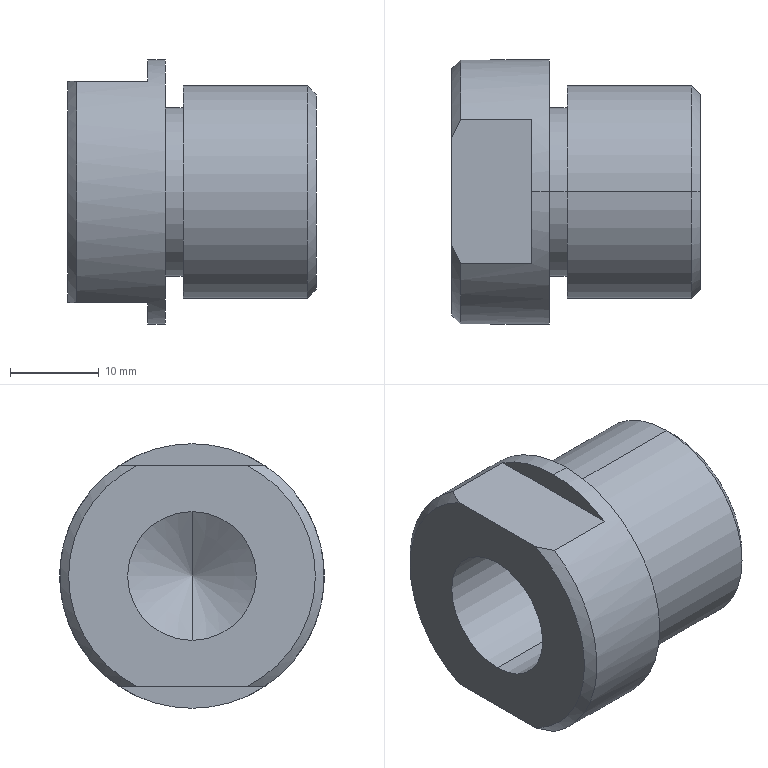Part | SolidWorks | features BaseBody 1 | 1 solid | 22 faces | box 28 x 29.8 x 29.8 mm | volume 11601 mm3 | cylinder 8 | plane 8 | cone 6 | commonest cylinder face diameters 14.5 x2 19 x2 24 x2 29.8 x2
STEP:
#1=CARTESIAN_POINT('',(27.,0.,12.));
#2=VERTEX_POINT('',#1);
#3=CARTESIAN_POINT('',(27.,0.,-12.));
#4=VERTEX_POINT('',#3);
#5=CARTESIAN_POINT('',(27.,0.,0.));
#6=DIRECTION('',(-1.,0.,0.));
#7=DIRECTION('',(0.,0.,1.));
#8=AXIS2_PLACEMENT_3D('',#5,#6,#7);
#9=CIRCLE('',#8,12.);
#10=EDGE_CURVE('',#2,#4,#9,.T.);
#11=ORIENTED_EDGE('',*,*,#10,.T.);
#12=CARTESIAN_POINT('',(13.,0.,-12.));
#13=VERTEX_POINT('',#12);
#14=CARTESIAN_POINT('',(0.,0.,-12.));
#15=DIRECTION('',(-1.,0.,0.));
#16=VECTOR('',#15,1000.);
#17=LINE('',#14,#16);
#18=EDGE_CURVE('',#4,#13,#17,.T.);
#19=ORIENTED_EDGE('',*,*,#18,.T.);
#20=CARTESIAN_POINT('',(13.,0.,12.));
#21=VERTEX_POINT('',#20);
#22=CARTESIAN_POINT('',(13.,0.,0.));
#23=DIRECTION('',(1.,0.,0.));
#24=DIRECTION('',(0.,0.,1.));
#25=AXIS2_PLACEMENT_3D('',#22,#23,#24);
#26=CIRCLE('',#25,12.);
#27=EDGE_CURVE('',#13,#21,#26,.T.);
#28=ORIENTED_EDGE('',*,*,#27,.T.);
#29=CARTESIAN_POINT('',(0.,0.,12.));
#30=DIRECTION('',(-1.,0.,0.));
#31=VECTOR('',#30,1000.);
#32=LINE('',#29,#31);
#33=EDGE_CURVE('',#2,#21,#32,.T.);
#34=ORIENTED_EDGE('',*,*,#33,.F.);
#35=EDGE_LOOP('',(#11,#19,#28,#34));
#36=FACE_OUTER_BOUND('',#35,.T.);
#37=CARTESIAN_POINT('',(0.,0.,0.));
#38=DIRECTION('',(-1.,0.,0.));
#39=DIRECTION('',(0.,0.,1.));
#40=AXIS2_PLACEMENT_3D('',#37,#38,#39);
#41=CYLINDRICAL_SURFACE('',#40,12.);
#42=ADVANCED_FACE('',(#36),#41,.T.);
#43=CARTESIAN_POINT('',(28.,0.,11.));
#44=VERTEX_POINT('',#43);
#45=CARTESIAN_POINT('',(28.,0.,-11.));
#46=VERTEX_POINT('',#45);
#47=CARTESIAN_POINT('',(28.,0.,0.));
#48=DIRECTION('',(-1.,0.,0.));
#49=DIRECTION('',(0.,0.,1.));
#50=AXIS2_PLACEMENT_3D('',#47,#48,#49);
#51=CIRCLE('',#50,11.);
#52=EDGE_CURVE('',#44,#46,#51,.T.);
#53=ORIENTED_EDGE('',*,*,#52,.T.);
#54=CARTESIAN_POINT('',(27.,0.,-12.));
#55=DIRECTION('',(-0.7071,0.,-0.7071));
#56=VECTOR('',#55,1000.);
#57=LINE('',#54,#56);
#58=EDGE_CURVE('',#46,#4,#57,.T.);
#59=ORIENTED_EDGE('',*,*,#58,.T.);
#60=ORIENTED_EDGE('',*,*,#10,.F.);
#61=CARTESIAN_POINT('',(27.,0.,12.));
#62=DIRECTION('',(-0.7071,0.,0.7071));
#63=VECTOR('',#62,1000.);
#64=LINE('',#61,#63);
#65=EDGE_CURVE('',#44,#2,#64,.T.);
#66=ORIENTED_EDGE('',*,*,#65,.F.);
#67=EDGE_LOOP('',(#53,#59,#60,#66));
#68=FACE_OUTER_BOUND('',#67,.T.);
#69=CARTESIAN_POINT('',(27.,0.,0.));
#70=DIRECTION('',(-1.,0.,0.));
#71=DIRECTION('',(0.,0.,1.));
#72=AXIS2_PLACEMENT_3D('',#69,#70,#71);
#73=CONICAL_SURFACE('',#72,12.,0.7854);
#74=ADVANCED_FACE('',(#68),#73,.T.);
#75=CARTESIAN_POINT('',(13.,0.,9.5));
#76=VERTEX_POINT('',#75);
#77=CARTESIAN_POINT('',(13.,0.,-9.5));
#78=VERTEX_POINT('',#77);
#79=CARTESIAN_POINT('',(13.,0.,0.));
#80=DIRECTION('',(-1.,0.,0.));
#81=DIRECTION('',(0.,0.,1.));
#82=AXIS2_PLACEMENT_3D('',#79,#80,#81);
#83=CIRCLE('',#82,9.5);
#84=EDGE_CURVE('',#76,#78,#83,.T.);
#85=ORIENTED_EDGE('',*,*,#84,.T.);
#86=CARTESIAN_POINT('',(11.,0.,-9.5));
#87=VERTEX_POINT('',#86);
#88=CARTESIAN_POINT('',(0.,0.,-9.5));
#89=DIRECTION('',(-1.,0.,0.));
#90=VECTOR('',#89,1000.);
#91=LINE('',#88,#90);
#92=EDGE_CURVE('',#78,#87,#91,.T.);
#93=ORIENTED_EDGE('',*,*,#92,.T.);
#94=CARTESIAN_POINT('',(11.,0.,9.5));
#95=VERTEX_POINT('',#94);
#96=CARTESIAN_POINT('',(11.,0.,0.));
#97=DIRECTION('',(1.,0.,0.));
#98=DIRECTION('',(0.,0.,1.));
#99=AXIS2_PLACEMENT_3D('',#96,#97,#98);
#100=CIRCLE('',#99,9.5);
#101=EDGE_CURVE('',#87,#95,#100,.T.);
#102=ORIENTED_EDGE('',*,*,#101,.T.);
#103=CARTESIAN_POINT('',(0.,0.,9.5));
#104=DIRECTION('',(-1.,0.,0.));
#105=VECTOR('',#104,1000.);
#106=LINE('',#103,#105);
#107=EDGE_CURVE('',#76,#95,#106,.T.);
#108=ORIENTED_EDGE('',*,*,#107,.F.);
#109=EDGE_LOOP('',(#85,#93,#102,#108));
#110=FACE_OUTER_BOUND('',#109,.T.);
#111=CARTESIAN_POINT('',(0.,0.,0.));
#112=DIRECTION('',(-1.,0.,0.));
#113=DIRECTION('',(0.,0.,1.));
#114=AXIS2_PLACEMENT_3D('',#111,#112,#113);
#115=CYLINDRICAL_SURFACE('',#114,9.5);
#116=ADVANCED_FACE('',(#110),#115,.T.);
#117=CARTESIAN_POINT('',(11.,0.,14.9));
#118=VERTEX_POINT('',#117);
#119=CARTESIAN_POINT('',(11.,0.,-14.9));
#120=VERTEX_POINT('',#119);
#121=CARTESIAN_POINT('',(11.,0.,0.));
#122=DIRECTION('',(-1.,0.,0.));
#123=DIRECTION('',(0.,0.,1.));
#124=AXIS2_PLACEMENT_3D('',#121,#122,#123);
#125=CIRCLE('',#124,14.9);
#126=EDGE_CURVE('',#118,#120,#125,.T.);
#127=ORIENTED_EDGE('',*,*,#126,.T.);
#128=CARTESIAN_POINT('',(9.,0.,-14.9));
#129=VERTEX_POINT('',#128);
#130=CARTESIAN_POINT('',(0.,0.,-14.9));
#131=DIRECTION('',(-1.,0.,0.));
#132=VECTOR('',#131,1000.);
#133=LINE('',#130,#132);
#134=EDGE_CURVE('',#120,#129,#133,.T.);
#135=ORIENTED_EDGE('',*,*,#134,.T.);
#136=CARTESIAN_POINT('',(9.,8.109,-12.5));
#137=VERTEX_POINT('',#136);
#138=CARTESIAN_POINT('',(9.,0.,0.));
#139=DIRECTION('',(1.,0.,0.));
#140=DIRECTION('',(0.,0.,1.));
#141=AXIS2_PLACEMENT_3D('',#138,#139,#140);
#142=CIRCLE('',#141,14.9);
#143=EDGE_CURVE('',#129,#137,#142,.T.);
#144=ORIENTED_EDGE('',*,*,#143,.T.);
#145=CARTESIAN_POINT('',(1.,8.109,-12.5));
#146=VERTEX_POINT('',#145);
#147=CARTESIAN_POINT('',(0.,8.109,-12.5));
#148=DIRECTION('',(-1.,0.,0.));
#149=VECTOR('',#148,1000.);
#150=LINE('',#147,#149);
#151=EDGE_CURVE('',#137,#146,#150,.T.);
#152=ORIENTED_EDGE('',*,*,#151,.T.);
#153=CARTESIAN_POINT('',(1.,8.109,12.5));
#154=VERTEX_POINT('',#153);
#155=CARTESIAN_POINT('',(1.,0.,0.));
#156=DIRECTION('',(1.,0.,0.));
#157=DIRECTION('',(0.,0.,1.));
#158=AXIS2_PLACEMENT_3D('',#155,#156,#157);
#159=CIRCLE('',#158,14.9);
#160=EDGE_CURVE('',#146,#154,#159,.T.);
#161=ORIENTED_EDGE('',*,*,#160,.T.);
#162=CARTESIAN_POINT('',(9.,8.109,12.5));
#163=VERTEX_POINT('',#162);
#164=CARTESIAN_POINT('',(0.,8.109,12.5));
#165=DIRECTION('',(1.,0.,0.));
#166=VECTOR('',#165,1000.);
#167=LINE('',#164,#166);
#168=EDGE_CURVE('',#154,#163,#167,.T.);
#169=ORIENTED_EDGE('',*,*,#168,.T.);
#170=CARTESIAN_POINT('',(9.,0.,14.9));
#171=VERTEX_POINT('',#170);
#172=CARTESIAN_POINT('',(9.,0.,0.));
#173=DIRECTION('',(1.,0.,0.));
#174=DIRECTION('',(0.,0.,1.));
#175=AXIS2_PLACEMENT_3D('',#172,#173,#174);
#176=CIRCLE('',#175,14.9);
#177=EDGE_CURVE('',#163,#171,#176,.T.);
#178=ORIENTED_EDGE('',*,*,#177,.T.);
#179=CARTESIAN_POINT('',(0.,0.,14.9));
#180=DIRECTION('',(-1.,0.,0.));
#181=VECTOR('',#180,1000.);
#182=LINE('',#179,#181);
#183=EDGE_CURVE('',#118,#171,#182,.T.);
#184=ORIENTED_EDGE('',*,*,#183,.F.);
#185=EDGE_LOOP('',(#127,#135,#144,#152,#161,#169,#178,#184));
#186=FACE_OUTER_BOUND('',#185,.T.);
#187=CARTESIAN_POINT('',(0.,0.,0.));
#188=DIRECTION('',(-1.,0.,0.));
#189=DIRECTION('',(0.,0.,1.));
#190=AXIS2_PLACEMENT_3D('',#187,#188,#189);
#191=CYLINDRICAL_SURFACE('',#190,14.9);
#192=ADVANCED_FACE('',(#186),#191,.T.);
#193=CARTESIAN_POINT('',(16.,0.,-7.25));
#194=VERTEX_POINT('',#193);
#195=CARTESIAN_POINT('',(16.,0.,7.25));
#196=VERTEX_POINT('',#195);
#197=CARTESIAN_POINT('',(16.,0.,0.));
#198=DIRECTION('',(-1.,0.,0.));
#199=DIRECTION('',(0.,0.,1.));
#200=AXIS2_PLACEMENT_3D('',#197,#198,#199);
#201=CIRCLE('',#200,7.25);
#202=EDGE_CURVE('',#194,#196,#201,.T.);
#203=ORIENTED_EDGE('',*,*,#202,.F.);
#204=CARTESIAN_POINT('',(0.,0.,-7.25));
#205=VERTEX_POINT('',#204);
#206=CARTESIAN_POINT('',(0.,0.,-7.25));
#207=DIRECTION('',(-1.,0.,0.));
#208=VECTOR('',#207,1000.);
#209=LINE('',#206,#208);
#210=EDGE_CURVE('',#194,#205,#209,.T.);
#211=ORIENTED_EDGE('',*,*,#210,.T.);
#212=CARTESIAN_POINT('',(0.,0.,7.25));
#213=VERTEX_POINT('',#212);
#214=CARTESIAN_POINT('',(0.,0.,0.));
#215=DIRECTION('',(-1.,0.,0.));
#216=DIRECTION('',(0.,0.,1.));
#217=AXIS2_PLACEMENT_3D('',#214,#215,#216);
#218=CIRCLE('',#217,7.25);
#219=EDGE_CURVE('',#205,#213,#218,.T.);
#220=ORIENTED_EDGE('',*,*,#219,.T.);
#221=CARTESIAN_POINT('',(0.,0.,7.25));
#222=DIRECTION('',(-1.,0.,0.));
#223=VECTOR('',#222,1000.);
#224=LINE('',#221,#223);
#225=EDGE_CURVE('',#196,#213,#224,.T.);
#226=ORIENTED_EDGE('',*,*,#225,.F.);
#227=EDGE_LOOP('',(#203,#211,#220,#226));
#228=FACE_OUTER_BOUND('',#227,.T.);
#229=CARTESIAN_POINT('',(0.,0.,0.));
#230=DIRECTION('',(-1.,0.,0.));
#231=DIRECTION('',(0.,0.,1.));
#232=AXIS2_PLACEMENT_3D('',#229,#230,#231);
#233=CYLINDRICAL_SURFACE('',#232,7.25);
#234=ADVANCED_FACE('',(#228),#233,.F.);
#235=CARTESIAN_POINT('',(20.356,0.,0.));
#236=VERTEX_POINT('',#235);
#237=CARTESIAN_POINT('',(16.,0.,7.25));
#238=DIRECTION('',(-0.515,0.,0.8572));
#239=VECTOR('',#238,1000.);
#240=LINE('',#237,#239);
#241=EDGE_CURVE('',#236,#196,#240,.T.);
#242=ORIENTED_EDGE('',*,*,#241,.F.);
#243=CARTESIAN_POINT('',(16.,0.,-7.25));
#244=DIRECTION('',(-0.515,0.,-0.8572));
#245=VECTOR('',#244,1000.);
#246=LINE('',#243,#245);
#247=EDGE_CURVE('',#236,#194,#246,.T.);
#248=ORIENTED_EDGE('',*,*,#247,.T.);
#249=ORIENTED_EDGE('',*,*,#202,.T.);
#250=EDGE_LOOP('',(#242,#248,#249));
#251=FACE_OUTER_BOUND('',#250,.T.);
#252=CARTESIAN_POINT('',(16.,0.,0.));
#253=DIRECTION('',(-1.,0.,0.));
#254=DIRECTION('',(0.,0.,1.));
#255=AXIS2_PLACEMENT_3D('',#252,#253,#254);
#256=CONICAL_SURFACE('',#255,7.25,1.03);
#257=ADVANCED_FACE('',(#251),#256,.F.);
#258=ORIENTED_EDGE('',*,*,#18,.F.);
#259=CARTESIAN_POINT('',(27.,0.,0.));
#260=DIRECTION('',(-1.,0.,0.));
#261=DIRECTION('',(0.,0.,1.));
#262=AXIS2_PLACEMENT_3D('',#259,#260,#261);
#263=CIRCLE('',#262,12.);
#264=EDGE_CURVE('',#4,#2,#263,.T.);
#265=ORIENTED_EDGE('',*,*,#264,.T.);
#266=ORIENTED_EDGE('',*,*,#33,.T.);
#267=CARTESIAN_POINT('',(13.,0.,0.));
#268=DIRECTION('',(1.,0.,0.));
#269=DIRECTION('',(0.,0.,1.));
#270=AXIS2_PLACEMENT_3D('',#267,#268,#269);
#271=CIRCLE('',#270,12.);
#272=EDGE_CURVE('',#21,#13,#271,.T.);
#273=ORIENTED_EDGE('',*,*,#272,.T.);
#274=EDGE_LOOP('',(#258,#265,#266,#273));
#275=FACE_OUTER_BOUND('',#274,.T.);
#276=CARTESIAN_POINT('',(0.,0.,0.));
#277=DIRECTION('',(-1.,0.,0.));
#278=DIRECTION('',(0.,0.,1.));
#279=AXIS2_PLACEMENT_3D('',#276,#277,#278);
#280=CYLINDRICAL_SURFACE('',#279,12.);
#281=ADVANCED_FACE('',(#275),#280,.T.);
#282=ORIENTED_EDGE('',*,*,#272,.F.);
#283=ORIENTED_EDGE('',*,*,#27,.F.);
#284=EDGE_LOOP('',(#282,#283));
#285=FACE_OUTER_BOUND('',#284,.T.);
#286=ORIENTED_EDGE('',*,*,#84,.F.);
#287=CARTESIAN_POINT('',(13.,0.,0.));
#288=DIRECTION('',(-1.,0.,0.));
#289=DIRECTION('',(0.,0.,1.));
#290=AXIS2_PLACEMENT_3D('',#287,#288,#289);
#291=CIRCLE('',#290,9.5);
#292=EDGE_CURVE('',#78,#76,#291,.T.);
#293=ORIENTED_EDGE('',*,*,#292,.F.);
#294=EDGE_LOOP('',(#286,#293));
#295=FACE_BOUND('',#294,.T.);
#296=CARTESIAN_POINT('',(13.,9.5,0.));
#297=DIRECTION('',(1.,0.,0.));
#298=DIRECTION('',(0.,0.,-1.));
#299=AXIS2_PLACEMENT_3D('',#296,#297,#298);
#300=PLANE('',#299);
#301=ADVANCED_FACE('',(#285,#295),#300,.F.);
#302=ORIENTED_EDGE('',*,*,#58,.F.);
#303=CARTESIAN_POINT('',(28.,0.,0.));
#304=DIRECTION('',(-1.,0.,0.));
#305=DIRECTION('',(0.,0.,1.));
#306=AXIS2_PLACEMENT_3D('',#303,#304,#305);
#307=CIRCLE('',#306,11.);
#308=EDGE_CURVE('',#46,#44,#307,.T.);
#309=ORIENTED_EDGE('',*,*,#308,.T.);
#310=ORIENTED_EDGE('',*,*,#65,.T.);
#311=ORIENTED_EDGE('',*,*,#264,.F.);
#312=EDGE_LOOP('',(#302,#309,#310,#311));
#313=FACE_OUTER_BOUND('',#312,.T.);
#314=CARTESIAN_POINT('',(27.,0.,0.));
#315=DIRECTION('',(-1.,0.,0.));
#316=DIRECTION('',(0.,0.,1.));
#317=AXIS2_PLACEMENT_3D('',#314,#315,#316);
#318=CONICAL_SURFACE('',#317,12.,0.7854);
#319=ADVANCED_FACE('',(#313),#318,.T.);
#320=ORIENTED_EDGE('',*,*,#92,.F.);
#321=ORIENTED_EDGE('',*,*,#292,.T.);
#322=ORIENTED_EDGE('',*,*,#107,.T.);
#323=CARTESIAN_POINT('',(11.,0.,0.));
#324=DIRECTION('',(1.,0.,0.));
#325=DIRECTION('',(0.,0.,1.));
#326=AXIS2_PLACEMENT_3D('',#323,#324,#325);
#327=CIRCLE('',#326,9.5);
#328=EDGE_CURVE('',#95,#87,#327,.T.);
#329=ORIENTED_EDGE('',*,*,#328,.T.);
#330=EDGE_LOOP('',(#320,#321,#322,#329));
#331=FACE_OUTER_BOUND('',#330,.T.);
#332=CARTESIAN_POINT('',(0.,0.,0.));
#333=DIRECTION('',(-1.,0.,0.));
#334=DIRECTION('',(0.,0.,1.));
#335=AXIS2_PLACEMENT_3D('',#332,#333,#334);
#336=CYLINDRICAL_SURFACE('',#335,9.5);
#337=ADVANCED_FACE('',(#331),#336,.T.);
#338=ORIENTED_EDGE('',*,*,#52,.F.);
#339=ORIENTED_EDGE('',*,*,#308,.F.);
#340=EDGE_LOOP('',(#338,#339));
#341=FACE_OUTER_BOUND('',#340,.T.);
#342=CARTESIAN_POINT('',(28.,12.,0.));
#343=DIRECTION('',(-1.,0.,0.));
#344=DIRECTION('',(0.,0.,1.));
#345=AXIS2_PLACEMENT_3D('',#342,#343,#344);
#346=PLANE('',#345);
#347=ADVANCED_FACE('',(#341),#346,.F.);
#348=ORIENTED_EDGE('',*,*,#328,.F.);
#349=ORIENTED_EDGE('',*,*,#101,.F.);
#350=EDGE_LOOP('',(#348,#349));
#351=FACE_BOUND('',#350,.T.);
#352=ORIENTED_EDGE('',*,*,#126,.F.);
#353=CARTESIAN_POINT('',(11.,0.,0.));
#354=DIRECTION('',(-1.,0.,0.));
#355=DIRECTION('',(0.,0.,1.));
#356=AXIS2_PLACEMENT_3D('',#353,#354,#355);
#357=CIRCLE('',#356,14.9);
#358=EDGE_CURVE('',#120,#118,#357,.T.);
#359=ORIENTED_EDGE('',*,*,#358,.F.);
#360=EDGE_LOOP('',(#352,#359));
#361=FACE_OUTER_BOUND('',#360,.T.);
#362=CARTESIAN_POINT('',(11.,14.9,0.));
#363=DIRECTION('',(-1.,0.,0.));
#364=DIRECTION('',(0.,0.,1.));
#365=AXIS2_PLACEMENT_3D('',#362,#363,#364);
#366=PLANE('',#365);
#367=ADVANCED_FACE('',(#351,#361),#366,.F.);
#368=ORIENTED_EDGE('',*,*,#134,.F.);
#369=ORIENTED_EDGE('',*,*,#358,.T.);
#370=ORIENTED_EDGE('',*,*,#183,.T.);
#371=CARTESIAN_POINT('',(9.,-8.109,12.5));
#372=VERTEX_POINT('',#371);
#373=CARTESIAN_POINT('',(9.,0.,0.));
#374=DIRECTION('',(1.,0.,0.));
#375=DIRECTION('',(0.,0.,1.));
#376=AXIS2_PLACEMENT_3D('',#373,#374,#375);
#377=CIRCLE('',#376,14.9);
#378=EDGE_CURVE('',#171,#372,#377,.T.);
#379=ORIENTED_EDGE('',*,*,#378,.T.);
#380=CARTESIAN_POINT('',(1.,-8.109,12.5));
#381=VERTEX_POINT('',#380);
#382=CARTESIAN_POINT('',(0.,-8.109,12.5));
#383=DIRECTION('',(-1.,0.,0.));
#384=VECTOR('',#383,1000.);
#385=LINE('',#382,#384);
#386=EDGE_CURVE('',#372,#381,#385,.T.);
#387=ORIENTED_EDGE('',*,*,#386,.T.);
#388=CARTESIAN_POINT('',(1.,-8.109,-12.5));
#389=VERTEX_POINT('',#388);
#390=CARTESIAN_POINT('',(1.,0.,0.));
#391=DIRECTION('',(1.,0.,0.));
#392=DIRECTION('',(0.,0.,1.));
#393=AXIS2_PLACEMENT_3D('',#390,#391,#392);
#394=CIRCLE('',#393,14.9);
#395=EDGE_CURVE('',#381,#389,#394,.T.);
#396=ORIENTED_EDGE('',*,*,#395,.T.);
#397=CARTESIAN_POINT('',(9.,-8.109,-12.5));
#398=VERTEX_POINT('',#397);
#399=CARTESIAN_POINT('',(0.,-8.109,-12.5));
#400=DIRECTION('',(1.,0.,0.));
#401=VECTOR('',#400,1000.);
#402=LINE('',#399,#401);
#403=EDGE_CURVE('',#389,#398,#402,.T.);
#404=ORIENTED_EDGE('',*,*,#403,.T.);
#405=CARTESIAN_POINT('',(9.,0.,0.));
#406=DIRECTION('',(1.,0.,0.));
#407=DIRECTION('',(0.,0.,1.));
#408=AXIS2_PLACEMENT_3D('',#405,#406,#407);
#409=CIRCLE('',#408,14.9);
#410=EDGE_CURVE('',#398,#129,#409,.T.);
#411=ORIENTED_EDGE('',*,*,#410,.T.);
#412=EDGE_LOOP('',(#368,#369,#370,#379,#387,#396,#404,#411));
#413=FACE_OUTER_BOUND('',#412,.T.);
#414=CARTESIAN_POINT('',(0.,0.,0.));
#415=DIRECTION('',(-1.,0.,0.));
#416=DIRECTION('',(0.,0.,1.));
#417=AXIS2_PLACEMENT_3D('',#414,#415,#416);
#418=CYLINDRICAL_SURFACE('',#417,14.9);
#419=ADVANCED_FACE('',(#413),#418,.T.);
#420=ORIENTED_EDGE('',*,*,#177,.F.);
#421=CARTESIAN_POINT('',(9.,0.,12.5));
#422=DIRECTION('',(0.,-1.,0.));
#423=VECTOR('',#422,1000.);
#424=LINE('',#421,#423);
#425=EDGE_CURVE('',#163,#372,#424,.T.);
#426=ORIENTED_EDGE('',*,*,#425,.T.);
#427=ORIENTED_EDGE('',*,*,#378,.F.);
#428=EDGE_LOOP('',(#420,#426,#427));
#429=FACE_OUTER_BOUND('',#428,.T.);
#430=CARTESIAN_POINT('',(9.,0.,0.));
#431=DIRECTION('',(-1.,0.,0.));
#432=DIRECTION('',(0.,0.,1.));
#433=AXIS2_PLACEMENT_3D('',#430,#431,#432);
#434=PLANE('',#433);
#435=ADVANCED_FACE('',(#429),#434,.T.);
#436=CARTESIAN_POINT('',(0.,-6.079,12.5));
#437=VERTEX_POINT('',#436);
#438=CARTESIAN_POINT('',(0.,6.079,12.5));
#439=VERTEX_POINT('',#438);
#440=CARTESIAN_POINT('',(0.,8.109,12.5));
#441=DIRECTION('',(0.,1.,0.));
#442=VECTOR('',#441,1000.);
#443=LINE('',#440,#442);
#444=EDGE_CURVE('',#437,#439,#443,.T.);
#445=ORIENTED_EDGE('',*,*,#444,.F.);
#446=CARTESIAN_POINT('',(1.,-8.109,12.5));
#447=CARTESIAN_POINT('',(0.6391,-7.446,12.5));
#448=CARTESIAN_POINT('',(0.3026,-6.771,12.5));
#449=CARTESIAN_POINT('',(0.,-6.079,12.5));
#450=B_SPLINE_CURVE_WITH_KNOTS('',3,(#446,#447,#448,#449),.UNSPECIFIED.,.F.,.F.,(4,4),(0.,0.002263),.UNSPECIFIED.);
#451=EDGE_CURVE('',#381,#437,#450,.T.);
#452=ORIENTED_EDGE('',*,*,#451,.F.);
#453=ORIENTED_EDGE('',*,*,#386,.F.);
#454=ORIENTED_EDGE('',*,*,#425,.F.);
#455=ORIENTED_EDGE('',*,*,#168,.F.);
#456=CARTESIAN_POINT('',(0.,6.079,12.5));
#457=CARTESIAN_POINT('',(0.3026,6.771,12.5));
#458=CARTESIAN_POINT('',(0.6391,7.446,12.5));
#459=CARTESIAN_POINT('',(1.,8.109,12.5));
#460=B_SPLINE_CURVE_WITH_KNOTS('',3,(#456,#457,#458,#459),.UNSPECIFIED.,.F.,.F.,(4,4),(0.,0.002263),.UNSPECIFIED.);
#461=EDGE_CURVE('',#439,#154,#460,.T.);
#462=ORIENTED_EDGE('',*,*,#461,.F.);
#463=EDGE_LOOP('',(#445,#452,#453,#454,#455,#462));
#464=FACE_OUTER_BOUND('',#463,.T.);
#465=CARTESIAN_POINT('',(9.,8.109,12.5));
#466=DIRECTION('',(0.,0.,-1.));
#467=DIRECTION('',(-1.,0.,0.));
#468=AXIS2_PLACEMENT_3D('',#465,#466,#467);
#469=PLANE('',#468);
#470=ADVANCED_FACE('',(#464),#469,.F.);
#471=CARTESIAN_POINT('',(0.,6.079,-12.5));
#472=VERTEX_POINT('',#471);
#473=CARTESIAN_POINT('',(1.,8.109,-12.5));
#474=CARTESIAN_POINT('',(0.6391,7.446,-12.5));
#475=CARTESIAN_POINT('',(0.3026,6.771,-12.5));
#476=CARTESIAN_POINT('',(0.,6.079,-12.5));
#477=B_SPLINE_CURVE_WITH_KNOTS('',3,(#473,#474,#475,#476),.UNSPECIFIED.,.F.,.F.,(4,4),(0.,0.002263),.UNSPECIFIED.);
#478=EDGE_CURVE('',#146,#472,#477,.T.);
#479=ORIENTED_EDGE('',*,*,#478,.T.);
#480=CARTESIAN_POINT('',(0.,0.,0.));
#481=DIRECTION('',(1.,0.,0.));
#482=DIRECTION('',(0.,0.,-1.));
#483=AXIS2_PLACEMENT_3D('',#480,#481,#482);
#484=CIRCLE('',#483,13.9);
#485=EDGE_CURVE('',#472,#439,#484,.T.);
#486=ORIENTED_EDGE('',*,*,#485,.T.);
#487=ORIENTED_EDGE('',*,*,#461,.T.);
#488=ORIENTED_EDGE('',*,*,#160,.F.);
#489=EDGE_LOOP('',(#479,#486,#487,#488));
#490=FACE_OUTER_BOUND('',#489,.T.);
#491=CARTESIAN_POINT('',(1.,0.,0.));
#492=DIRECTION('',(1.,0.,0.));
#493=DIRECTION('',(0.,0.,-1.));
#494=AXIS2_PLACEMENT_3D('',#491,#492,#493);
#495=CONICAL_SURFACE('',#494,14.9,0.7854);
#496=ADVANCED_FACE('',(#490),#495,.T.);
#497=CARTESIAN_POINT('',(0.,-6.079,-12.5));
#498=VERTEX_POINT('',#497);
#499=CARTESIAN_POINT('',(0.,8.109,-12.5));
#500=DIRECTION('',(0.,-1.,0.));
#501=VECTOR('',#500,1000.);
#502=LINE('',#499,#501);
#503=EDGE_CURVE('',#472,#498,#502,.T.);
#504=ORIENTED_EDGE('',*,*,#503,.F.);
#505=ORIENTED_EDGE('',*,*,#478,.F.);
#506=ORIENTED_EDGE('',*,*,#151,.F.);
#507=CARTESIAN_POINT('',(9.,8.109,-12.5));
#508=DIRECTION('',(0.,1.,0.));
#509=VECTOR('',#508,1000.);
#510=LINE('',#507,#509);
#511=EDGE_CURVE('',#398,#137,#510,.T.);
#512=ORIENTED_EDGE('',*,*,#511,.F.);
#513=ORIENTED_EDGE('',*,*,#403,.F.);
#514=CARTESIAN_POINT('',(0.,-6.079,-12.5));
#515=CARTESIAN_POINT('',(0.3026,-6.771,-12.5));
#516=CARTESIAN_POINT('',(0.6391,-7.446,-12.5));
#517=CARTESIAN_POINT('',(1.,-8.109,-12.5));
#518=B_SPLINE_CURVE_WITH_KNOTS('',3,(#514,#515,#516,#517),.UNSPECIFIED.,.F.,.F.,(4,4),(0.,0.002263),.UNSPECIFIED.);
#519=EDGE_CURVE('',#498,#389,#518,.T.);
#520=ORIENTED_EDGE('',*,*,#519,.F.);
#521=EDGE_LOOP('',(#504,#505,#506,#512,#513,#520));
#522=FACE_OUTER_BOUND('',#521,.T.);
#523=CARTESIAN_POINT('',(9.,8.109,-12.5));
#524=DIRECTION('',(0.,0.,1.));
#525=DIRECTION('',(1.,0.,0.));
#526=AXIS2_PLACEMENT_3D('',#523,#524,#525);
#527=PLANE('',#526);
#528=ADVANCED_FACE('',(#522),#527,.F.);
#529=ORIENTED_EDGE('',*,*,#410,.F.);
#530=ORIENTED_EDGE('',*,*,#511,.T.);
#531=ORIENTED_EDGE('',*,*,#143,.F.);
#532=EDGE_LOOP('',(#529,#530,#531));
#533=FACE_OUTER_BOUND('',#532,.T.);
#534=CARTESIAN_POINT('',(9.,0.,0.));
#535=DIRECTION('',(-1.,0.,0.));
#536=DIRECTION('',(0.,0.,1.));
#537=AXIS2_PLACEMENT_3D('',#534,#535,#536);
#538=PLANE('',#537);
#539=ADVANCED_FACE('',(#533),#538,.T.);
#540=ORIENTED_EDGE('',*,*,#519,.T.);
#541=ORIENTED_EDGE('',*,*,#395,.F.);
#542=ORIENTED_EDGE('',*,*,#451,.T.);
#543=CARTESIAN_POINT('',(0.,0.,0.));
#544=DIRECTION('',(1.,0.,0.));
#545=DIRECTION('',(0.,0.,-1.));
#546=AXIS2_PLACEMENT_3D('',#543,#544,#545);
#547=CIRCLE('',#546,13.9);
#548=EDGE_CURVE('',#437,#498,#547,.T.);
#549=ORIENTED_EDGE('',*,*,#548,.T.);
#550=EDGE_LOOP('',(#540,#541,#542,#549));
#551=FACE_OUTER_BOUND('',#550,.T.);
#552=CARTESIAN_POINT('',(1.,0.,0.));
#553=DIRECTION('',(1.,0.,0.));
#554=DIRECTION('',(0.,0.,-1.));
#555=AXIS2_PLACEMENT_3D('',#552,#553,#554);
#556=CONICAL_SURFACE('',#555,14.9,0.7854);
#557=ADVANCED_FACE('',(#551),#556,.T.);
#558=CARTESIAN_POINT('',(0.,0.,0.));
#559=DIRECTION('',(-1.,0.,0.));
#560=DIRECTION('',(0.,0.,1.));
#561=AXIS2_PLACEMENT_3D('',#558,#559,#560);
#562=CIRCLE('',#561,7.25);
#563=EDGE_CURVE('',#213,#205,#562,.T.);
#564=ORIENTED_EDGE('',*,*,#563,.F.);
#565=ORIENTED_EDGE('',*,*,#219,.F.);
#566=EDGE_LOOP('',(#564,#565));
#567=FACE_BOUND('',#566,.T.);
#568=ORIENTED_EDGE('',*,*,#444,.T.);
#569=ORIENTED_EDGE('',*,*,#485,.F.);
#570=ORIENTED_EDGE('',*,*,#503,.T.);
#571=ORIENTED_EDGE('',*,*,#548,.F.);
#572=EDGE_LOOP('',(#568,#569,#570,#571));
#573=FACE_OUTER_BOUND('',#572,.T.);
#574=CARTESIAN_POINT('',(0.,0.,0.));
#575=DIRECTION('',(1.,0.,0.));
#576=DIRECTION('',(0.,0.,-1.));
#577=AXIS2_PLACEMENT_3D('',#574,#575,#576);
#578=PLANE('',#577);
#579=ADVANCED_FACE('',(#567,#573),#578,.F.);
#580=ORIENTED_EDGE('',*,*,#210,.F.);
#581=CARTESIAN_POINT('',(16.,0.,0.));
#582=DIRECTION('',(-1.,0.,0.));
#583=DIRECTION('',(0.,0.,1.));
#584=AXIS2_PLACEMENT_3D('',#581,#582,#583);
#585=CIRCLE('',#584,7.25);
#586=EDGE_CURVE('',#196,#194,#585,.T.);
#587=ORIENTED_EDGE('',*,*,#586,.F.);
#588=ORIENTED_EDGE('',*,*,#225,.T.);
#589=ORIENTED_EDGE('',*,*,#563,.T.);
#590=EDGE_LOOP('',(#580,#587,#588,#589));
#591=FACE_OUTER_BOUND('',#590,.T.);
#592=CARTESIAN_POINT('',(0.,0.,0.));
#593=DIRECTION('',(-1.,0.,0.));
#594=DIRECTION('',(0.,0.,1.));
#595=AXIS2_PLACEMENT_3D('',#592,#593,#594);
#596=CYLINDRICAL_SURFACE('',#595,7.25);
#597=ADVANCED_FACE('',(#591),#596,.F.);
#598=ORIENTED_EDGE('',*,*,#247,.F.);
#599=ORIENTED_EDGE('',*,*,#241,.T.);
#600=ORIENTED_EDGE('',*,*,#586,.T.);
#601=EDGE_LOOP('',(#598,#599,#600));
#602=FACE_OUTER_BOUND('',#601,.T.);
#603=CARTESIAN_POINT('',(16.,0.,0.));
#604=DIRECTION('',(-1.,0.,0.));
#605=DIRECTION('',(0.,0.,1.));
#606=AXIS2_PLACEMENT_3D('',#603,#604,#605);
#607=CONICAL_SURFACE('',#606,7.25,1.03);
#608=ADVANCED_FACE('',(#602),#607,.F.);
#609=CLOSED_SHELL('',(#42,#74,#116,#192,#234,#257,#281,#301,#319,#337,#347,#367,#419,#435,#470,#496,#528,#539,#557,#579,#597,#608));
#610=MANIFOLD_SOLID_BREP('',#609);
#611=CARTESIAN_POINT('',(0.,0.,0.));
#612=DIRECTION('',(0.,0.,1.));
#613=DIRECTION('',(1.,0.,0.));
#614=AXIS2_PLACEMENT_3D('',#611,#612,#613);
#615=(LENGTH_UNIT()NAMED_UNIT(*)SI_UNIT(.MILLI.,.METRE.));
#616=UNCERTAINTY_MEASURE_WITH_UNIT(LENGTH_MEASURE(0.00001),#615,'','');
#617=(NAMED_UNIT(*)PLANE_ANGLE_UNIT()SI_UNIT($,.RADIAN.));
#618=(NAMED_UNIT(*)SI_UNIT($,.STERADIAN.)SOLID_ANGLE_UNIT());
#619=(GEOMETRIC_REPRESENTATION_CONTEXT(3)GLOBAL_UNCERTAINTY_ASSIGNED_CONTEXT((#616))GLOBAL_UNIT_ASSIGNED_CONTEXT((#615,#617,#618))REPRESENTATION_CONTEXT('',''));
#620=ADVANCED_BREP_SHAPE_REPRESENTATION('',(#610,#614),#619);